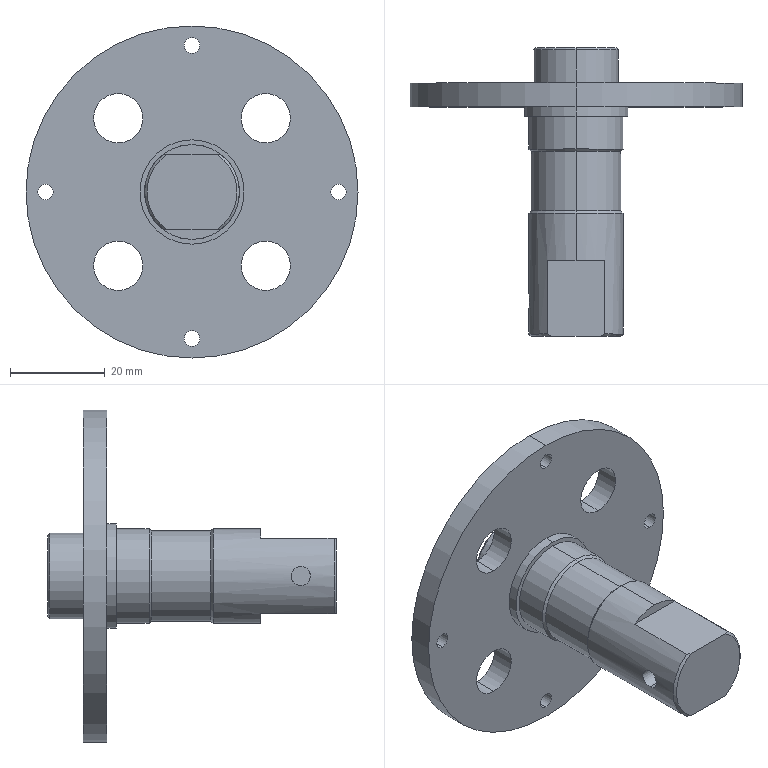Part | SolidWorks | features ICE 9, Chamfer 2, HoleWzd 2, Extrusion 1 | 1 solid | 52 faces | box 70 x 60.9 x 70 mm | volume 33459 mm3 | cylinder 32 | cone 10 | plane 10 | commonest cylinder face diameters 3.3 x10 10.4 x8 20 x4 4 x2 18 x2 19 x2